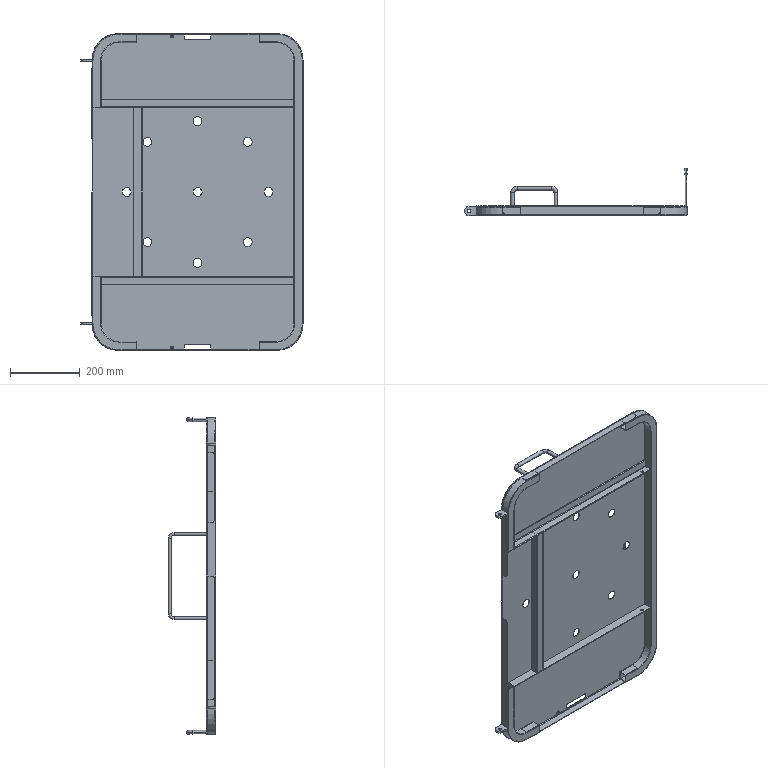Part | NX | features BREP 9 | 12 solids | 362 faces | box 638.529 x 135.642 x 910.285 mm | volume 1497627 mm3 | plane 174 | cylinder 148 | torus 28 | spline 12 | commonest cylinder face diameters 3.175 x45 25.4 x20 11.113 x12 7.938 x10 19.05 x10 10.998 x8